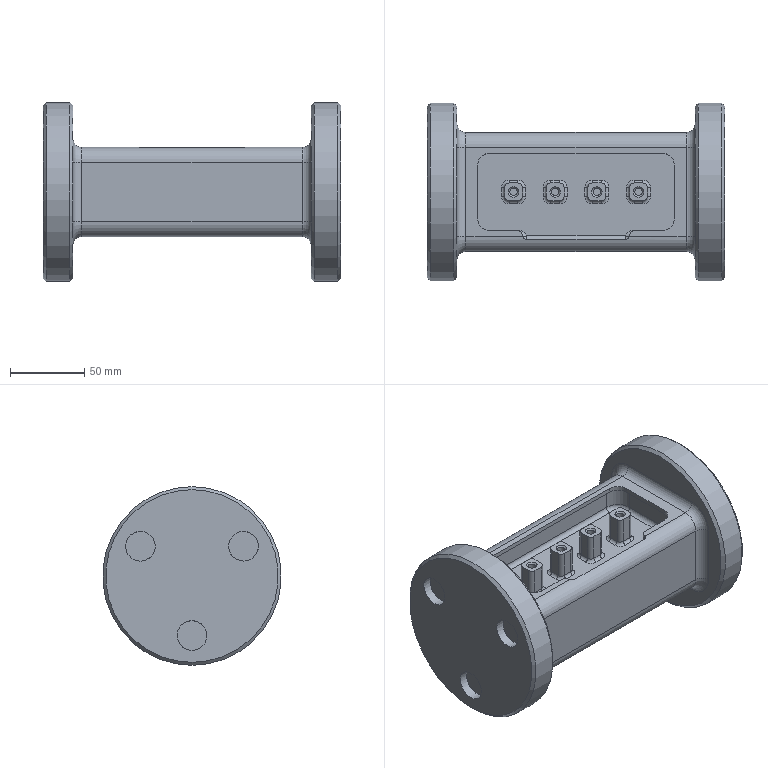NC program | NX | posted with a generic post | part box 200 x 120 x 120 mm
Lines 1 to 1228 of 4340:
N10 G17 G21 G94 G90
(PLANAR_MILL , TOOL : PD)
N12 T00 M6
N14 G53
N16 G17 G0 G90 X-59. Y-54. S4000 M3
N18 G43 Z40. H0
N20 Z3.
N22 G94 G1 Z0. F1000.
N24 Y-30.
N26 Y30.
N28 X-35.4
N30 Y-30.
N32 X-11.8
N34 Y30.
N36 X11.8
N38 Y-30.
N40 X35.4
N42 Y30.
N44 X59.
N46 Y-30.
N48 Y-54.
N50 Z3.
N52 G0 Z40.
N54 M5
(CAVITY_MILL , TOOL : D12R1)
N56 T01 M6
N58 G53
N60 G17 G0 G90 X-3.568 Y-10.163 S0 M3
N62 G43 Z40. H1
N64 Z-1.69
N66 G94 G3 X0. Y-13.85 Z-1.99 R3.57 F250.
N68 G1 X24.242
N70 G2 X25.721 Y-12.538 R21.15
N72 X24.359 Y-10.278 R16.35
N74 X17. Y-13.35 R10.35
N76 G1 X11.
N78 G2 X0.65 Y-3. R10.35
N80 G1 Y3.
N82 G2 X1.857 Y7.85 R10.35
N84 G1 X2.917 Y7.288
N86 G2 X11. Y12.15 R9.15
N88 G1 X17.
N90 G2 X26.15 Y3. R9.15
N92 G1 Y-3.
N94 G2 X17. Y-12.15 R9.15
N96 G1 X11.
N98 G2 X1.85 Y-3. R9.15
N100 G1 Y3.
N102 G2 X2.917 Y7.288 R9.15
N104 G1 X1.857 Y7.85
N106 X-1.857
N108 G2 X-0.65 Y3. R10.35
N110 G1 Y-3.
N112 G2 X-11. Y-13.35 R10.35
N114 G1 X-17.
N116 G2 X-24.359 Y-10.278 R10.35
N118 G1 X-23.506 Y-9.434
N120 G2 X-26.15 Y-3. R9.15
N122 G1 Y3.
N124 G2 X-17. Y12.15 R9.15
N126 G1 X-11.
N128 G2 X-1.85 Y3. R9.15
N130 G1 Y-3.
N132 G2 X-11. Y-12.15 R9.15
N134 G1 X-17.
N136 G2 X-23.506 Y-9.434 R9.15
N138 G1 X-24.359 Y-10.278
N140 G2 X-25.721 Y-12.538 R16.35
N142 X-24.242 Y-13.85 R21.15
N144 G1 X0.
N146 Y-19.85
N148 X26.925
N150 G2 X39. Y-13.85 R15.15
N152 G1 X53.85
N154 Y-8.367
N156 G2 X45. Y-13.35 R10.35
N158 G1 X39.
N160 G2 X28.65 Y-3. R10.35
N162 G1 Y3.
N164 G2 X39. Y13.35 R10.35
N166 G1 X45.
N168 G2 X53.85 Y8.367 R10.35
N170 G1 X52.824 Y7.744
N172 G2 X54.15 Y3. R9.15
N174 G1 Y-3.
N176 G2 X45. Y-12.15 R9.15
N178 G1 X39.
N180 G2 X29.85 Y-3. R9.15
N182 G1 Y3.
N184 G2 X39. Y12.15 R9.15
N186 G1 X45.
N188 G2 X52.824 Y7.744 R9.15
N190 G1 X53.85 Y8.367
N192 Y13.85
N194 X-53.85
N196 Y8.367
N198 G2 X-45. Y13.35 R10.35
N200 G1 X-39.
N202 G2 X-28.65 Y3. R10.35
N204 G1 Y-3.
N206 G2 X-39. Y-13.35 R10.35
N208 G1 X-45.
N210 G2 X-53.85 Y-8.367 R10.35
N212 G1 X-52.824 Y-7.744
N214 G2 X-54.15 Y-3. R9.15
N216 G1 Y3.
N218 G2 X-45. Y12.15 R9.15
N220 G1 X-39.
N222 G2 X-29.85 Y3. R9.15
N224 G1 Y-3.
N226 G2 X-39. Y-12.15 R9.15
N228 G1 X-45.
N230 G2 X-52.824 Y-7.744 R9.15
N232 G1 X-53.85 Y-8.367
N234 Y-13.85
N236 X-39.
N238 G2 X-26.925 Y-19.85 R15.15
N240 G1 X0.
N242 Y-25.85
N244 X30.409
N246 G2 X39. Y-19.85 R9.15
N248 G1 X58.
N250 G3 X59.85 Y-18. R1.85
N252 G1 Y18.
N254 G3 X58. Y19.85 R1.85
N256 G1 X-58.
N258 G3 X-59.85 Y18. R1.85
N260 G1 Y-18.
N262 G3 X-58. Y-19.85 R1.85
N264 G1 X-39.
N266 G2 X-30.409 Y-25.85 R9.15
N268 G1 X0.
N270 Z-1.69
N272 G0 Z40.
N274 X-3.568 Y-10.163
N276 Z-3.68
N278 G3 X0. Y-13.85 Z-3.98 R3.57
N280 G1 X24.242
N282 G2 X25.721 Y-12.538 R21.15
N284 X24.359 Y-10.278 R16.35
N286 X17. Y-13.35 R10.35
N288 G1 X11.
N290 G2 X0.65 Y-3. R10.35
N292 G1 Y3.
N294 G2 X1.857 Y7.85 R10.35
N296 G1 X2.917 Y7.288
N298 G2 X11. Y12.15 R9.15
N300 G1 X17.
N302 G2 X26.15 Y3. R9.15
N304 G1 Y-3.
N306 G2 X17. Y-12.15 R9.15
N308 G1 X11.
N310 G2 X1.85 Y-3. R9.15
N312 G1 Y3.
N314 G2 X2.917 Y7.288 R9.15
N316 G1 X1.857 Y7.85
N318 X-1.857
N320 G2 X-0.65 Y3. R10.35
N322 G1 Y-3.
N324 G2 X-11. Y-13.35 R10.35
N326 G1 X-17.
N328 G2 X-24.359 Y-10.278 R10.35
N330 G1 X-23.506 Y-9.434
N332 G2 X-26.15 Y-3. R9.15
N334 G1 Y3.
N336 G2 X-17. Y12.15 R9.15
N338 G1 X-11.
N340 G2 X-1.85 Y3. R9.15
N342 G1 Y-3.
N344 G2 X-11. Y-12.15 R9.15
N346 G1 X-17.
N348 G2 X-23.506 Y-9.434 R9.15
N350 G1 X-24.359 Y-10.278
N352 G2 X-25.721 Y-12.538 R16.35
N354 X-24.242 Y-13.85 R21.15
N356 G1 X0.
N358 Y-19.85
N360 X26.925
N362 G2 X39. Y-13.85 R15.15
N364 G1 X53.85
N366 Y-8.367
N368 G2 X45. Y-13.35 R10.35
N370 G1 X39.
N372 G2 X28.65 Y-3. R10.35
N374 G1 Y3.
N376 G2 X39. Y13.35 R10.35
N378 G1 X45.
N380 G2 X53.85 Y8.367 R10.35
N382 G1 X52.824 Y7.744
N384 G2 X54.15 Y3. R9.15
N386 G1 Y-3.
N388 G2 X45. Y-12.15 R9.15
N390 G1 X39.
N392 G2 X29.85 Y-3. R9.15
N394 G1 Y3.
N396 G2 X39. Y12.15 R9.15
N398 G1 X45.
N400 G2 X52.824 Y7.744 R9.15
N402 G1 X53.85 Y8.367
N404 Y13.85
N406 X-53.85
N408 Y8.367
N410 G2 X-45. Y13.35 R10.35
N412 G1 X-39.
N414 G2 X-28.65 Y3. R10.35
N416 G1 Y-3.
N418 G2 X-39. Y-13.35 R10.35
N420 G1 X-45.
N422 G2 X-53.85 Y-8.367 R10.35
N424 G1 X-52.824 Y-7.744
N426 G2 X-54.15 Y-3. R9.15
N428 G1 Y3.
N430 G2 X-45. Y12.15 R9.15
N432 G1 X-39.
N434 G2 X-29.85 Y3. R9.15
N436 G1 Y-3.
N438 G2 X-39. Y-12.15 R9.15
N440 G1 X-45.
N442 G2 X-52.824 Y-7.744 R9.15
N444 G1 X-53.85 Y-8.367
N446 Y-13.85
N448 X-39.
N450 G2 X-26.925 Y-19.85 R15.15
N452 G1 X0.
N454 Y-25.85
N456 X30.409
N458 G2 X39. Y-19.85 R9.15
N460 G1 X58.
N462 G3 X59.85 Y-18. R1.85
N464 G1 Y18.
N466 G3 X58. Y19.85 R1.85
N468 G1 X-58.
N470 G3 X-59.85 Y18. R1.85
N472 G1 Y-18.
N474 G3 X-58. Y-19.85 R1.85
N476 G1 X-39.
N478 G2 X-30.409 Y-25.85 R9.15
N480 G1 X0.
N482 Z-3.68
N484 G0 Z-1.69
N486 X-3.568 Y-10.163
N488 Z-5.67
N490 G3 X0. Y-13.85 Z-5.97 R3.57
N492 G1 X24.242
N494 G2 X25.721 Y-12.538 R21.15
N496 X24.359 Y-10.278 R16.35
N498 X17. Y-13.35 R10.35
N500 G1 X11.
N502 G2 X0.65 Y-3. R10.35
N504 G1 Y3.
N506 G2 X1.857 Y7.85 R10.35
N508 G1 X2.917 Y7.288
N510 G2 X11. Y12.15 R9.15
N512 G1 X17.
N514 G2 X26.15 Y3. R9.15
N516 G1 Y-3.
N518 G2 X17. Y-12.15 R9.15
N520 G1 X11.
N522 G2 X1.85 Y-3. R9.15
N524 G1 Y3.
N526 G2 X2.917 Y7.288 R9.15
N528 G1 X1.857 Y7.85
N530 X-1.857
N532 G2 X-0.65 Y3. R10.35
N534 G1 Y-3.
N536 G2 X-11. Y-13.35 R10.35
N538 G1 X-17.
N540 G2 X-24.359 Y-10.278 R10.35
N542 G1 X-23.506 Y-9.434
N544 G2 X-26.15 Y-3. R9.15
N546 G1 Y3.
N548 G2 X-17. Y12.15 R9.15
N550 G1 X-11.
N552 G2 X-1.85 Y3. R9.15
N554 G1 Y-3.
N556 G2 X-11. Y-12.15 R9.15
N558 G1 X-17.
N560 G2 X-23.506 Y-9.434 R9.15
N562 G1 X-24.359 Y-10.278
N564 G2 X-25.721 Y-12.538 R16.35
N566 X-24.242 Y-13.85 R21.15
N568 G1 X0.
N570 Y-19.85
N572 X26.925
N574 G2 X39. Y-13.85 R15.15
N576 G1 X53.85
N578 Y-8.367
N580 G2 X45. Y-13.35 R10.35
N582 G1 X39.
N584 G2 X28.65 Y-3. R10.35
N586 G1 Y3.
N588 G2 X39. Y13.35 R10.35
N590 G1 X45.
N592 G2 X53.85 Y8.367 R10.35
N594 G1 X52.824 Y7.744
N596 G2 X54.15 Y3. R9.15
N598 G1 Y-3.
N600 G2 X45. Y-12.15 R9.15
N602 G1 X39.
N604 G2 X29.85 Y-3. R9.15
N606 G1 Y3.
N608 G2 X39. Y12.15 R9.15
N610 G1 X45.
N612 G2 X52.824 Y7.744 R9.15
N614 G1 X53.85 Y8.367
N616 Y13.85
N618 X-53.85
N620 Y8.367
N622 G2 X-45. Y13.35 R10.35
N624 G1 X-39.
N626 G2 X-28.65 Y3. R10.35
N628 G1 Y-3.
N630 G2 X-39. Y-13.35 R10.35
N632 G1 X-45.
N634 G2 X-53.85 Y-8.367 R10.35
N636 G1 X-52.824 Y-7.744
N638 G2 X-54.15 Y-3. R9.15
N640 G1 Y3.
N642 G2 X-45. Y12.15 R9.15
N644 G1 X-39.
N646 G2 X-29.85 Y3. R9.15
N648 G1 Y-3.
N650 G2 X-39. Y-12.15 R9.15
N652 G1 X-45.
N654 G2 X-52.824 Y-7.744 R9.15
N656 G1 X-53.85 Y-8.367
N658 Y-13.85
N660 X-39.
N662 G2 X-26.925 Y-19.85 R15.15
N664 G1 X0.
N666 Y-25.85
N668 X30.409
N670 G2 X39. Y-19.85 R9.15
N672 G1 X57.963
N674 G3 X59.85 Y-17.919 R1.855
N676 G1 Y17.919
N678 G3 X57.963 Y19.85 R1.855
N680 G1 X-57.963
N682 G3 X-59.85 Y17.919 R1.855
N684 G1 Y-17.919
N686 G3 X-57.963 Y-19.85 R1.855
N688 G1 X-39.
N690 G2 X-30.409 Y-25.85 R9.15
N692 G1 X0.
N694 Z-5.67
N696 G0 Z-3.68
N698 X-3.568 Y-10.163
N700 Z-7.66
N702 G3 X0. Y-13.85 Z-7.96 R3.57
N704 G1 X24.242
N706 G2 X25.721 Y-12.538 R21.15
N708 X24.359 Y-10.278 R16.35
N710 X17. Y-13.35 R10.35
N712 G1 X11.
N714 G2 X0.65 Y-3. R10.35
N716 G1 Y3.
N718 G2 X1.857 Y7.85 R10.35
N720 G1 X2.917 Y7.288
N722 G2 X11. Y12.15 R9.15
N724 G1 X17.
N726 G2 X26.15 Y3. R9.15
N728 G1 Y-3.
N730 G2 X17. Y-12.15 R9.15
N732 G1 X11.
N734 G2 X1.85 Y-3. R9.15
N736 G1 Y3.
N738 G2 X2.917 Y7.288 R9.15
N740 G1 X1.857 Y7.85
N742 X-1.857
N744 G2 X-0.65 Y3. R10.35
N746 G1 Y-3.
N748 G2 X-11. Y-13.35 R10.35
N750 G1 X-17.
N752 G2 X-24.359 Y-10.278 R10.35
N754 G1 X-23.506 Y-9.434
N756 G2 X-26.15 Y-3. R9.15
N758 G1 Y3.
N760 G2 X-17. Y12.15 R9.15
N762 G1 X-11.
N764 G2 X-1.85 Y3. R9.15
N766 G1 Y-3.
N768 G2 X-11. Y-12.15 R9.15
N770 G1 X-17.
N772 G2 X-23.506 Y-9.434 R9.15
N774 G1 X-24.359 Y-10.278
N776 G2 X-25.721 Y-12.538 R16.35
N778 X-24.242 Y-13.85 R21.15
N780 G1 X0.
N782 Y-19.85
N784 X26.925
N786 G2 X39. Y-13.85 R15.15
N788 G1 X53.85
N790 Y-8.367
N792 G2 X45. Y-13.35 R10.35
N794 G1 X39.
N796 G2 X28.65 Y-3. R10.35
N798 G1 Y3.
N800 G2 X39. Y13.35 R10.35
N802 G1 X45.
N804 G2 X53.85 Y8.367 R10.35
N806 G1 X52.824 Y7.744
N808 G2 X54.15 Y3. R9.15
N810 G1 Y-3.
N812 G2 X45. Y-12.15 R9.15
N814 G1 X39.
N816 G2 X29.85 Y-3. R9.15
N818 G1 Y3.
N820 G2 X39. Y12.15 R9.15
N822 G1 X45.
N824 G2 X52.824 Y7.744 R9.15
N826 G1 X53.85 Y8.367
N828 Y13.85
N830 X-53.85
N832 Y8.367
N834 G2 X-45. Y13.35 R10.35
N836 G1 X-39.
N838 G2 X-28.65 Y3. R10.35
N840 G1 Y-3.
N842 G2 X-39. Y-13.35 R10.35
N844 G1 X-45.
N846 G2 X-53.85 Y-8.367 R10.35
N848 G1 X-52.824 Y-7.744
N850 G2 X-54.15 Y-3. R9.15
N852 G1 Y3.
N854 G2 X-45. Y12.15 R9.15
N856 G1 X-39.
N858 G2 X-29.85 Y3. R9.15
N860 G1 Y-3.
N862 G2 X-39. Y-12.15 R9.15
N864 G1 X-45.
N866 G2 X-52.824 Y-7.744 R9.15
N868 G1 X-53.85 Y-8.367
N870 Y-13.85
N872 X-39.
N874 G2 X-26.925 Y-19.85 R15.15
N876 G1 X0.
N878 Y-25.85
N880 X30.409
N882 G2 X39. Y-19.85 R9.15
N884 G1 X57.963
N886 G3 X59.85 Y-17.919 R1.855
N888 G1 Y17.919
N890 G3 X57.963 Y19.85 R1.855
N892 G1 X-57.963
N894 G3 X-59.85 Y17.919 R1.855
N896 G1 Y-17.919
N898 G3 X-57.963 Y-19.85 R1.855
N900 G1 X-39.
N902 G2 X-30.409 Y-25.85 R9.15
N904 G1 X0.
N906 Z-7.66
N908 G0 Z-5.67
N910 X-3.568 Y-10.163
N912 Z-9.65
N914 G3 X0. Y-13.85 Z-9.95 R3.57
N916 G1 X24.242
N918 G2 X25.721 Y-12.538 R21.15
N920 X24.359 Y-10.278 R16.35
N922 X17. Y-13.35 R10.35
N924 G1 X11.
N926 G2 X0.65 Y-3. R10.35
N928 G1 Y3.
N930 G2 X1.857 Y7.85 R10.35
N932 G1 X2.917 Y7.288
N934 G2 X11. Y12.15 R9.15
N936 G1 X17.
N938 G2 X26.15 Y3. R9.15
N940 G1 Y-3.
N942 G2 X17. Y-12.15 R9.15
N944 G1 X11.
N946 G2 X1.85 Y-3. R9.15
N948 G1 Y3.
N950 G2 X2.917 Y7.288 R9.15
N952 G1 X1.857 Y7.85
N954 X-1.857
N956 G2 X-0.65 Y3. R10.35
N958 G1 Y-3.
N960 G2 X-11. Y-13.35 R10.35
N962 G1 X-17.
N964 G2 X-24.359 Y-10.278 R10.35
N966 G1 X-23.506 Y-9.434
N968 G2 X-26.15 Y-3. R9.15
N970 G1 Y3.
N972 G2 X-17. Y12.15 R9.15
N974 G1 X-11.
N976 G2 X-1.85 Y3. R9.15
N978 G1 Y-3.
N980 G2 X-11. Y-12.15 R9.15
N982 G1 X-17.
N984 G2 X-23.506 Y-9.434 R9.15
N986 G1 X-24.359 Y-10.278
N988 G2 X-25.721 Y-12.538 R16.35
N990 X-24.242 Y-13.85 R21.15
N992 G1 X0.
N994 Y-19.85
N996 X26.925
N998 G2 X39. Y-13.85 R15.15
N1000 G1 X53.85
N1002 Y-8.367
N1004 G2 X45. Y-13.35 R10.35
N1006 G1 X39.
N1008 G2 X28.65 Y-3. R10.35
N1010 G1 Y3.
N1012 G2 X39. Y13.35 R10.35
N1014 G1 X45.
N1016 G2 X53.85 Y8.367 R10.35
N1018 G1 X52.824 Y7.744
N1020 G2 X54.15 Y3. R9.15
N1022 G1 Y-3.
N1024 G2 X45. Y-12.15 R9.15
N1026 G1 X39.
N1028 G2 X29.85 Y-3. R9.15
N1030 G1 Y3.
N1032 G2 X39. Y12.15 R9.15
N1034 G1 X45.
N1036 G2 X52.824 Y7.744 R9.15
N1038 G1 X53.85 Y8.367
N1040 Y13.85
N1042 X-53.85
N1044 Y8.367
N1046 G2 X-45. Y13.35 R10.35
N1048 G1 X-39.
N1050 G2 X-28.65 Y3. R10.35
N1052 G1 Y-3.
N1054 G2 X-39. Y-13.35 R10.35
N1056 G1 X-45.
N1058 G2 X-53.85 Y-8.367 R10.35
N1060 G1 X-52.824 Y-7.744
N1062 G2 X-54.15 Y-3. R9.15
N1064 G1 Y3.
N1066 G2 X-45. Y12.15 R9.15
N1068 G1 X-39.
N1070 G2 X-29.85 Y3. R9.15
N1072 G1 Y-3.
N1074 G2 X-39. Y-12.15 R9.15
N1076 G1 X-45.
N1078 G2 X-52.824 Y-7.744 R9.15
N1080 G1 X-53.85 Y-8.367
N1082 Y-13.85
N1084 X-39.
N1086 G2 X-26.925 Y-19.85 R15.15
N1088 G1 X0.
N1090 Y-25.85
N1092 X30.409
N1094 G2 X39. Y-19.85 R9.15
N1096 G1 X57.963
N1098 G3 X59.85 Y-17.919 R1.855
N1100 G1 Y17.919
N1102 G3 X57.963 Y19.85 R1.855
N1104 G1 X-57.963
N1106 G3 X-59.85 Y17.919 R1.855
N1108 G1 Y-17.919
N1110 G3 X-57.963 Y-19.85 R1.855
N1112 G1 X-39.
N1114 G2 X-30.409 Y-25.85 R9.15
N1116 G1 X0.
N1118 Z-9.65
N1120 G0 Z-7.66
N1122 X-3.568 Y-10.163
N1124 Z-11.64
N1126 G3 X0. Y-13.85 Z-11.94 R3.57
N1128 G1 X24.242
N1130 G2 X25.721 Y-12.538 R21.15
N1132 X24.359 Y-10.278 R16.35
N1134 X17. Y-13.35 R10.35
N1136 G1 X11.
N1138 G2 X0.65 Y-3. R10.35
N1140 G1 Y3.
N1142 G2 X1.857 Y7.85 R10.35
N1144 G1 X2.917 Y7.288
N1146 G2 X11. Y12.15 R9.15
N1148 G1 X17.
N1150 G2 X26.15 Y3. R9.15
N1152 G1 Y-3.
N1154 G2 X17. Y-12.15 R9.15
N1156 G1 X11.
N1158 G2 X1.85 Y-3. R9.15
N1160 G1 Y3.
N1162 G2 X2.917 Y7.288 R9.15
N1164 G1 X1.857 Y7.85
N1166 X-1.857
N1168 G2 X-0.65 Y3. R10.35
N1170 G1 Y-3.
N1172 G2 X-11. Y-13.35 R10.35
N1174 G1 X-17.
N1176 G2 X-24.359 Y-10.278 R10.35
N1178 G1 X-23.506 Y-9.434
N1180 G2 X-26.15 Y-3. R9.15
N1182 G1 Y3.
N1184 G2 X-17. Y12.15 R9.15
N1186 G1 X-11.
N1188 G2 X-1.85 Y3. R9.15
N1190 G1 Y-3.
N1192 G2 X-11. Y-12.15 R9.15
N1194 G1 X-17.
N1196 G2 X-23.506 Y-9.434 R9.15
N1198 G1 X-24.359 Y-10.278
N1200 G2 X-25.721 Y-12.538 R16.35
N1202 X-24.242 Y-13.85 R21.15
N1204 G1 X0.
N1206 Y-19.85
N1208 X26.925
N1210 G2 X39. Y-13.85 R15.15
N1212 G1 X53.85
N1214 Y-8.367
N1216 G2 X45. Y-13.35 R10.35
N1218 G1 X39.
N1220 G2 X28.65 Y-3. R10.35
N1222 G1 Y3.
N1224 G2 X39. Y13.35 R10.35
N1226 G1 X45.
N1228 G2 X53.85 Y8.367 R10.35
N1230 G1 X52.824 Y7.744
N1232 G2 X54.15 Y3. R9.15
N1234 G1 Y-3.
N1236 G2 X45. Y-12.15 R9.15
N1238 G1 X39.
N1240 G2 X29.85 Y-3. R9.15
N1242 G1 Y3.
N1244 G2 X39. Y12.15 R9.15
N1246 G1 X45.
N1248 G2 X52.824 Y7.744 R9.15
N1250 G1 X53.85 Y8.367
N1252 Y13.85
N1254 X-53.85
N1256 Y8.367
N1258 G2 X-45. Y13.35 R10.35
N1260 G1 X-39.
N1262 G2 X-28.65 Y3. R10.35
N1264 G1 Y-3.
N1266 G2 X-39. Y-13.35 R10.35
N1268 G1 X-45.
N1270 G2 X-53.85 Y-8.367 R10.35
N1272 G1 X-52.824 Y-7.744
N1274 G2 X-54.15 Y-3. R9.15
N1276 G1 Y3.
N1278 G2 X-45. Y12.15 R9.15
N1280 G1 X-39.
N1282 G2 X-29.85 Y3. R9.15
N1284 G1 Y-3.
N1286 G2 X-39. Y-12.15 R9.15
N1288 G1 X-45.
N1290 G2 X-52.824 Y-7.744 R9.15
N1292 G1 X-53.85 Y-8.367
N1294 Y-13.85
N1296 X-39.
N1298 G2 X-26.925 Y-19.85 R15.15
N1300 G1 X0.
N1302 Y-25.85
N1304 X30.409
N1306 G2 X39. Y-19.85 R9.15
N1308 G1 X57.963
N1310 G3 X59.85 Y-17.919 R1.856
N1312 G1 Y17.919
N1314 G3 X57.963 Y19.85 R1.856
N1316 G1 X-57.963
N1318 G3 X-59.85 Y17.919 R1.856
N1320 G1 Y-17.919
N1322 G3 X-57.963 Y-19.85 R1.856
N1324 G1 X-39.
N1326 G2 X-30.409 Y-25.85 R9.15
N1328 G1 X0.
N1330 Z-11.64
N1332 G0 Z-9.65
N1334 X-3.568 Y-10.163
N1336 Z-13.63
N1338 G3 X0. Y-13.85 Z-13.93 R3.57
N1340 G1 X24.242
N1342 G2 X25.721 Y-12.538 R21.15
N1344 X24.359 Y-10.278 R16.35
N1346 X17. Y-13.35 R10.35
N1348 G1 X11.
N1350 G2 X0.65 Y-3. R10.35
N1352 G1 Y3.
N1354 G2 X1.857 Y7.85 R10.35
N1356 G1 X2.917 Y7.288
N1358 G2 X11. Y12.15 R9.15
N1360 G1 X17.
N1362 G2 X26.15 Y3. R9.15
N1364 G1 Y-3.
N1366 G2 X17. Y-12.15 R9.15
N1368 G1 X11.
N1370 G2 X1.85 Y-3. R9.15
N1372 G1 Y3.
N1374 G2 X2.917 Y7.288 R9.15
N1376 G1 X1.857 Y7.85
N1378 X-1.857
N1380 G2 X-0.65 Y3. R10.35
N1382 G1 Y-3.
N1384 G2 X-11. Y-13.35 R10.35
N1386 G1 X-17.
N1388 G2 X-24.359 Y-10.278 R10.35
N1390 G1 X-23.506 Y-9.434
N1392 G2 X-26.15 Y-3. R9.15
N1394 G1 Y3.
N1396 G2 X-17. Y12.15 R9.15
N1398 G1 X-11.
N1400 G2 X-1.85 Y3. R9.15
N1402 G1 Y-3.
N1404 G2 X-11. Y-12.15 R9.15
N1406 G1 X-17.
N1408 G2 X-23.506 Y-9.434 R9.15
N1410 G1 X-24.359 Y-10.278
N1412 G2 X-25.721 Y-12.538 R16.35
N1414 X-24.242 Y-13.85 R21.15
N1416 G1 X0.
N1418 Y-19.85
N1420 X26.925
N1422 G2 X39. Y-13.85 R15.15
N1424 G1 X53.85
N1426 Y-8.367
N1428 G2 X45. Y-13.35 R10.35
N1430 G1 X39.
N1432 G2 X28.65 Y-3. R10.35
N1434 G1 Y3.
N1436 G2 X39. Y13.35 R10.35
N1438 G1 X45.
N1440 G2 X53.85 Y8.367 R10.35
N1442 G1 X52.824 Y7.744
N1444 G2 X54.15 Y3. R9.15
N1446 G1 Y-3.
N1448 G2 X45. Y-12.15 R9.15
N1450 G1 X39.
N1452 G2 X29.85 Y-3. R9.15
N1454 G1 Y3.
N1456 G2 X39. Y12.15 R9.15
N1458 G1 X45.
N1460 G2 X52.824 Y7.744 R9.15
N1462 G1 X53.85 Y8.367
N1464 Y13.85
N1466 X-53.85
N1468 Y8.367
N1470 G2 X-45. Y13.35 R10.35
N1472 G1 X-39.
N1474 G2 X-28.65 Y3. R10.35
N1476 G1 Y-3.
N1478 G2 X-39. Y-13.35 R10.35
N1480 G1 X-45.
N1482 G2 X-53.85 Y-8.367 R10.35
N1484 G1 X-52.824 Y-7.744
N1486 G2 X-54.15 Y-3. R9.15
N1488 G1 Y3.
N1490 G2 X-45. Y12.15 R9.15
N1492 G1 X-39.
N1494 G2 X-29.85 Y3. R9.15
N1496 G1 Y-3.
N1498 G2 X-39. Y-12.15 R9.15
N1500 G1 X-45.
N1502 G2 X-52.824 Y-7.744 R9.15
N1504 G1 X-53.85 Y-8.367
N1506 Y-13.85
N1508 X-39.
N1510 G2 X-26.925 Y-19.85 R15.15
N1512 G1 X0.
N1514 Y-25.85
N1516 X30.409
N1518 G2 X39. Y-19.85 R9.15
N1520 G1 X57.963
N1522 G3 X59.85 Y-17.919 R1.856
N1524 G1 Y17.919
N1526 G3 X57.963 Y19.85 R1.856
N1528 G1 X-57.963
N1530 G3 X-59.85 Y17.919 R1.856
N1532 G1 Y-17.919
N1534 G3 X-57.963 Y-19.85 R1.856
N1536 G1 X-39.
N1538 G2 X-30.409 Y-25.85 R9.15
N1540 G1 X0.
N1542 Z-13.63
N1544 G0 Z-11.64
N1546 X-3.568 Y-10.163
N1548 Z-15.62
N1550 G3 X0. Y-13.85 Z-15.92 R3.57
N1552 G1 X24.242
N1554 G2 X25.721 Y-12.538 R21.15
N1556 X24.359 Y-10.278 R16.35
N1558 X17. Y-13.35 R10.35
N1560 G1 X11.
N1562 G2 X0.65 Y-3. R10.35
N1564 G1 Y3.
N1566 G2 X1.857 Y7.85 R10.35
N1568 G1 X2.917 Y7.288
N1570 G2 X11. Y12.15 R9.15
N1572 G1 X17.
N1574 G2 X26.15 Y3. R9.15
N1576 G1 Y-3.
N1578 G2 X17. Y-12.15 R9.15
N1580 G1 X11.
N1582 G2 X1.85 Y-3. R9.15
N1584 G1 Y3.
N1586 G2 X2.917 Y7.288 R9.15
N1588 G1 X1.857 Y7.85
N1590 X-1.857
N1592 G2 X-0.65 Y3. R10.35
N1594 G1 Y-3.
N1596 G2 X-11. Y-13.35 R10.35
N1598 G1 X-17.
N1600 G2 X-24.359 Y-10.278 R10.35
N1602 G1 X-23.506 Y-9.434
N1604 G2 X-26.15 Y-3. R9.15
N1606 G1 Y3.
N1608 G2 X-17. Y12.15 R9.15
N1610 G1 X-11.
N1612 G2 X-1.85 Y3. R9.15
N1614 G1 Y-3.
N1616 G2 X-11. Y-12.15 R9.15
N1618 G1 X-17.
N1620 G2 X-23.506 Y-9.434 R9.15
N1622 G1 X-24.359 Y-10.278
N1624 G2 X-25.721 Y-12.538 R16.35
N1626 X-24.242 Y-13.85 R21.15
N1628 G1 X0.
N1630 Y-19.85
N1632 X26.925
N1634 G2 X39. Y-13.85 R15.15
N1636 G1 X53.85
N1638 Y-8.367
N1640 G2 X45. Y-13.35 R10.35
N1642 G1 X39.
N1644 G2 X28.65 Y-3. R10.35
N1646 G1 Y3.
N1648 G2 X39. Y13.35 R10.35
N1650 G1 X45.
N1652 G2 X53.85 Y8.367 R10.35
N1654 G1 X52.824 Y7.744
N1656 G2 X54.15 Y3. R9.15
N1658 G1 Y-3.
N1660 G2 X45. Y-12.15 R9.15
N1662 G1 X39.
N1664 G2 X29.85 Y-3. R9.15
N1666 G1 Y3.
N1668 G2 X39. Y12.15 R9.15
N1670 G1 X45.
N1672 G2 X52.824 Y7.744 R9.15
N1674 G1 X53.85 Y8.367
N1676 Y13.85
N1678 X-53.85
N1680 Y8.367
N1682 G2 X-45. Y13.35 R10.35
N1684 G1 X-39.
N1686 G2 X-28.65 Y3. R10.35
N1688 G1 Y-3.
N1690 G2 X-39. Y-13.35 R10.35
N1692 G1 X-45.
N1694 G2 X-53.85 Y-8.367 R10.35
N1696 G1 X-52.824 Y-7.744
N1698 G2 X-54.15 Y-3. R9.15
N1700 G1 Y3.
N1702 G2 X-45. Y12.15 R9.15
N1704 G1 X-39.
N1706 G2 X-29.85 Y3. R9.15
N1708 G1 Y-3.
N1710 G2 X-39. Y-12.15 R9.15
N1712 G1 X-45.
N1714 G2 X-52.824 Y-7.744 R9.15
N1716 G1 X-53.85 Y-8.367
N1718 Y-13.85
N1720 X-39.
N1722 G2 X-26.925 Y-19.85 R15.15
N1724 G1 X0.
N1726 Y-25.85
N1728 X30.409
N1730 G2 X39. Y-19.85 R9.15
N1732 G1 X57.963
N1734 G3 X59.85 Y-17.919 R1.857
N1736 G1 Y17.919
N1738 G3 X57.963 Y19.85 R1.857
N1740 G1 X-57.963
N1742 G3 X-59.85 Y17.919 R1.857
N1744 G1 Y-17.919
N1746 G3 X-57.963 Y-19.85 R1.857
N1748 G1 X-39.
N1750 G2 X-30.409 Y-25.85 R9.15
N1752 G1 X0.
N1754 Z-15.62
N1756 G0 Z-13.63
N1758 X-3.568 Y-10.163
N1760 Z-17.61
N1762 G3 X0. Y-13.85 Z-17.91 R3.57
N1764 G1 X24.242
N1766 G2 X25.721 Y-12.538 R21.15
N1768 X24.359 Y-10.278 R16.35
N1770 X17. Y-13.35 R10.35
N1772 G1 X11.
N1774 G2 X0.65 Y-3. R10.35
N1776 G1 Y3.
N1778 G2 X1.857 Y7.85 R10.35
N1780 G1 X2.917 Y7.288
N1782 G2 X11. Y12.15 R9.15
N1784 G1 X17.
N1786 G2 X26.15 Y3. R9.15
N1788 G1 Y-3.
N1790 G2 X17. Y-12.15 R9.15
N1792 G1 X11.
N1794 G2 X1.85 Y-3. R9.15
N1796 G1 Y3.
N1798 G2 X2.917 Y7.288 R9.15
N1800 G1 X1.857 Y7.85
N1802 X-1.857
N1804 G2 X-0.65 Y3. R10.35
N1806 G1 Y-3.
N1808 G2 X-11. Y-13.35 R10.35
N1810 G1 X-17.
N1812 G2 X-24.359 Y-10.278 R10.35
N1814 G1 X-23.506 Y-9.434
N1816 G2 X-26.15 Y-3. R9.15
N1818 G1 Y3.
N1820 G2 X-17. Y12.15 R9.15
N1822 G1 X-11.
N1824 G2 X-1.85 Y3. R9.15
N1826 G1 Y-3.
N1828 G2 X-11. Y-12.15 R9.15
N1830 G1 X-17.
N1832 G2 X-23.506 Y-9.434 R9.15
N1834 G1 X-24.359 Y-10.278
N1836 G2 X-25.721 Y-12.538 R16.35
N1838 X-24.242 Y-13.85 R21.15
N1840 G1 X0.
N1842 Y-19.85
N1844 X26.925
N1846 G2 X39. Y-13.85 R15.15
N1848 G1 X53.85
N1850 Y-8.367
N1852 G2 X45. Y-13.35 R10.35
N1854 G1 X39.
N1856 G2 X28.65 Y-3. R10.35
N1858 G1 Y3.
N1860 G2 X39. Y13.35 R10.35
N1862 G1 X45.
N1864 G2 X53.85 Y8.367 R10.35
N1866 G1 X52.824 Y7.744
N1868 G2 X54.15 Y3. R9.15
N1870 G1 Y-3.
N1872 G2 X45. Y-12.15 R9.15
N1874 G1 X39.
N1876 G2 X29.85 Y-3. R9.15
N1878 G1 Y3.
N1880 G2 X39. Y12.15 R9.15
N1882 G1 X45.
N1884 G2 X52.824 Y7.744 R9.15
N1886 G1 X53.85 Y8.367
N1888 Y13.85
N1890 X-53.85
N1892 Y8.367
N1894 G2 X-45. Y13.35 R10.35
N1896 G1 X-39.
N1898 G2 X-28.65 Y3. R10.35
N1900 G1 Y-3.
N1902 G2 X-39. Y-13.35 R10.35
N1904 G1 X-45.
N1906 G2 X-53.85 Y-8.367 R10.35
N1908 G1 X-52.824 Y-7.744
N1910 G2 X-54.15 Y-3. R9.15
N1912 G1 Y3.
N1914 G2 X-45. Y12.15 R9.15
N1916 G1 X-39.
N1918 G2 X-29.85 Y3. R9.15
N1920 G1 Y-3.
N1922 G2 X-39. Y-12.15 R9.15
N1924 G1 X-45.
N1926 G2 X-52.824 Y-7.744 R9.15
N1928 G1 X-53.85 Y-8.367
N1930 Y-13.85
N1932 X-39.
N1934 G2 X-26.925 Y-19.85 R15.15
N1936 G1 X0.
N1938 Y-25.85
N1940 X30.409
N1942 G2 X39. Y-19.85 R9.15
N1944 G1 X57.963
N1946 G3 X59.85 Y-17.919 R1.857
N1948 G1 Y17.919
N1950 G3 X57.963 Y19.85 R1.857
N1952 G1 X-57.963
N1954 G3 X-59.85 Y17.919 R1.857
N1956 G1 Y-17.919
N1958 G3 X-57.963 Y-19.85 R1.857
N1960 G1 X-39.
N1962 G2 X-30.409 Y-25.85 R9.15
N1964 G1 X0.
N1966 Z-17.61
N1968 G0 Z-15.62
N1970 X-3.879 Y-14.62
N1972 Z-19.6
N1974 G3 X0. Y-18.119 Z-19.9 R3.9
N1976 G1 X28.459
N1978 G2 X37.096 Y-13.97 R15.15
N1980 G1 X42.305 Y-14.513
N1982 X37.096 Y-13.97
N1984 G2 X28. Y-4.723 R11.134
N1986 G1 X29.186 Y-4.537
N1988 G2 X29.066 Y-3. R9.934
N1990 G1 Y3.
N1992 G2 X39. Y12.934 R9.934
N1994 G1 X45.
N1996 G2 X54.934 Y3. R9.934
N1998 G1 Y-3.
N2000 G2 X45. Y-12.934 R9.934
N2002 G1 X39.
N2004 G2 X29.186 Y-4.537 R9.934
N2006 G1 X28. Y-4.723
N2008 G2 X17. Y-14.134 R11.134
N2010 G1 X11.
N2012 G2 X0. Y-4.723 R11.134
N2014 G1 X1.186 Y-4.537
N2016 G2 X1.066 Y-3. R9.934
N2018 G1 Y3.
N2020 G2 X11. Y12.934 R9.934
N2022 G1 X17.
N2024 G2 X26.934 Y3. R9.934
N2026 G1 Y-3.
N2028 G2 X17. Y-12.934 R9.934
N2030 G1 X11.
N2032 G2 X1.186 Y-4.537 R9.934
N2034 G1 X0. Y-4.723
N2036 G2 X-11. Y-14.134 R11.134
N2038 G1 X-17.
N2040 G2 X-28. Y-4.723 R11.134
N2042 G1 X-26.814 Y-4.537
N2044 G2 X-26.934 Y-3. R9.934
N2046 G1 Y3.
N2048 G2 X-17. Y12.934 R9.934
N2050 G1 X-11.
N2052 G2 X-1.066 Y3. R9.934
N2054 G1 Y-3.
N2056 G2 X-11. Y-12.934 R9.934
N2058 G1 X-17.
N2060 G2 X-26.814 Y-4.537 R9.934
N2062 G1 X-28. Y-4.723
N2064 G2 X-37.096 Y-13.97 R11.134
N2066 G1 X-42.305 Y-14.513
N2068 X-37.096 Y-13.97
N2070 X-37.301 Y-12.788
N2072 G2 X-39. Y-12.934 R9.934
N2074 G1 X-45.
N2076 G2 X-54.934 Y-3. R9.934
N2078 G1 Y3.
N2080 G2 X-45. Y12.934 R9.934
N2082 G1 X-39.
N2084 G2 X-29.066 Y3. R9.934
N2086 G1 Y-3.
N2088 G2 X-37.301 Y-12.788 R9.934
N2090 G1 X-37.096 Y-13.97
N2092 G2 X-28.459 Y-18.119 R15.15
N2094 G1 X0.
N2096 Y-24.119
N2098 X30.694
N2100 G2 X32.108 Y-22.981 R10.881
N2102 X39. Y-19.85 R9.15
N2104 G1 X47.499
N2106 Y-13.85
N2108 X53.85
N2110 Y-9.756
N2112 G2 X47.499 Y-13.85 R11.134
N2114 G1 Y-19.85
N2116 X57.963
N2118 G3 X59.85 Y-17.919 R1.857
N2120 G1 Y9.756
N2122 X53.85
N2124 Y13.85
N2126 X47.499
N2128 X42. Y14.502
N2130 X47.499 Y13.85
N2132 G2 X53.85 Y9.756 R11.134
N2134 G1 X59.85
N2136 Y17.919
N2138 G3 X57.963 Y19.85 R1.858
N2140 G1 X36.501
N2142 Y13.85
N2144 X19.499
N2146 X14. Y14.502
N2148 X19.499 Y13.85
N2150 G2 X28. Y4.723 R11.134
N2152 X36.501 Y13.85 R11.134
N2154 G1 Y19.85
N2156 X8.501
N2158 Y13.85
N2160 X-8.501
N2162 X-14. Y14.502
N2164 X-8.501 Y13.85
N2166 G2 X0. Y4.723 R11.134
N2168 X8.501 Y13.85 R11.134
N2170 G1 Y19.85
N2172 X-19.499
N2174 Y13.85
N2176 X-36.501
N2178 X-42. Y14.502
N2180 X-36.501 Y13.85
N2182 G2 X-28. Y4.723 R11.134
N2184 X-19.499 Y13.85 R11.134
N2186 G1 Y19.85
N2188 X-47.499
N2190 Y13.85
N2192 X-53.85
N2194 Y9.756
N2196 G2 X-47.499 Y13.85 R11.134
N2198 G1 Y19.85
N2200 X-57.963
N2202 G3 X-59.85 Y17.919 R1.857
N2204 G1 Y-9.756
N2206 X-53.85
N2208 Y-13.85
N2210 X-47.499
N2212 G2 X-53.85 Y-9.756 R11.134
N2214 G1 X-59.85
N2216 Y-17.919
N2218 G3 X-57.963 Y-19.85 R1.858
N2220 G1 X-39.
N2222 G2 X-32.108 Y-22.981 R9.15
N2224 X-30.694 Y-24.119 R10.881
N2226 G1 X0.
N2228 Z-19.6
N2230 G0 Z40.
N2232 M5
(PLANAR_MILL_1 , TOOL : D10)
N2234 T00 M6
N2236 G53
N2238 G17 G0 G90 X-2.827 Y-16.853 S0 M3
N2240 G43 Z40. H0
N2242 Z-19.7
N2244 G94 G3 X0. Y-18.5 Z-20. R3.25 F250.
N2246 G1 X28.709
N2248 G2 X38.196 Y-15.5 R16.5
N2250 G1 X55.5
N2252 Y-6.6
N2254 G2 X45. Y-14.1 R11.1
N2256 G1 X39.
N2258 G2 X28. Y-4.487 R11.1
N2260 G1 X29.09 Y-4.339
N2262 G2 X29. Y-3. R10.
N2264 G1 Y3.
N2266 G2 X39. Y13. R10.
N2268 G1 X45.
N2270 G2 X55. Y3. R10.
N2272 G1 Y-3.
N2274 G2 X45. Y-13. R10.
N2276 G1 X39.
N2278 G2 X29.09 Y-4.339 R10.
N2280 G1 X28. Y-4.487
N2282 G2 X17. Y-14.1 R11.1
N2284 G1 X11.
N2286 G2 X0. Y-4.487 R11.1
N2288 G1 X1.09 Y-4.339
N2290 G2 X1. Y-3. R10.
N2292 G1 Y3.
N2294 G2 X11. Y13. R10.
N2296 G1 X17.
N2298 G2 X27. Y3. R10.
N2300 G1 Y-3.
N2302 G2 X17. Y-13. R10.
N2304 G1 X11.
N2306 G2 X1.09 Y-4.339 R10.
N2308 G1 X0. Y-4.487
N2310 G2 X-11. Y-14.1 R11.1
N2312 G1 X-17.
N2314 G2 X-28. Y-4.487 R11.1
N2316 G1 X-26.91 Y-4.339
N2318 G2 X-27. Y-3. R10.
N2320 G1 Y3.
N2322 G2 X-17. Y13. R10.
N2324 G1 X-11.
N2326 G2 X-1. Y3. R10.
N2328 G1 Y-3.
N2330 G2 X-11. Y-13. R10.
N2332 G1 X-17.
N2334 G2 X-26.91 Y-4.339 R10.
N2336 G1 X-28. Y-4.487
N2338 G2 X-39. Y-14.1 R11.1
N2340 G1 X-45.
N2342 G2 X-55.5 Y-6.6 R11.1
N2344 G1 X-54.459 Y-6.243
N2346 G2 X-55. Y-3. R10.
N2348 G1 Y3.
N2350 G2 X-45. Y13. R10.
N2352 G1 X-39.
N2354 G2 X-29. Y3. R10.
N2356 G1 Y-3.
N2358 G2 X-39. Y-13. R10.
N2360 G1 X-45.
N2362 G2 X-54.459 Y-6.243 R10.
N2364 G1 X-55.5 Y-6.6
N2366 Y-15.5
N2368 X-38.196
N2370 G2 X-28.709 Y-18.5 R16.5
N2372 G1 X0.
N2374 Y-24.
N2376 X30.646
N2378 G2 X38.196 Y-21. R11.
N2380 G1 X58.
N2382 G3 X61. Y-18. R3.
N2384 G1 Y6.6
N2386 X55.5
N2388 Y15.5
N2390 X-55.5
N2392 Y6.6
N2394 G2 X-45. Y14.1 R11.1
N2396 G1 X-39.
N2398 G2 X-28. Y4.487 R11.1
N2400 X-17. Y14.1 R11.1
N2402 G1 X-11.
N2404 G2 X0. Y4.487 R11.1
N2406 X11. Y14.1 R11.1
N2408 G1 X17.
N2410 G2 X28. Y4.487 R11.1
N2412 X39. Y14.1 R11.1
N2414 G1 X45.
N2416 G2 X55.5 Y6.6 R11.1
N2418 G1 X61.
N2420 Y18.
N2422 G3 X58. Y21. R3.
N2424 G1 X-58.
N2426 G3 X-61. Y18. R3.
N2428 G1 Y-18.
N2430 G3 X-58. Y-21. R3.
N2432 G1 X-38.196
N2434 G2 X-30.646 Y-24. R11.
N2436 G1 X0.
N2438 Z-19.7
N2440 G0 Z40.
N2442 M5